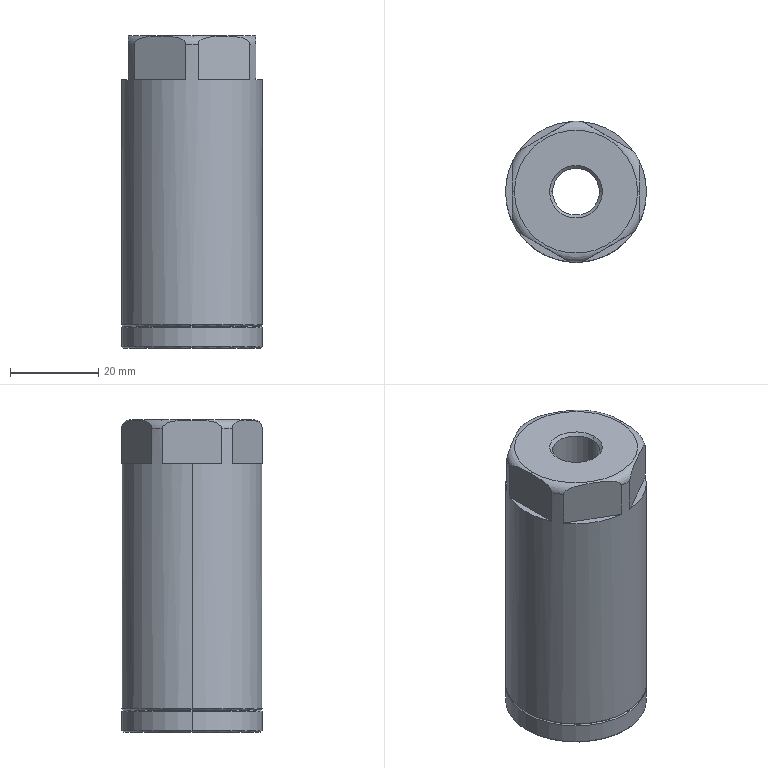Part | SolidWorks | features BaseBody 1 | 1 solid | 35 faces | box 32 x 32 x 71 mm | volume 42303 mm3 | plane 15 | cone 10 | cylinder 8 | torus 2 | commonest cylinder face diameters 10.647 x2 16.5 x2 31.9 x2 32 x2
STEP:
#1=CARTESIAN_POINT('',(-749.081,681.211,947.532));
#2=VERTEX_POINT('',#1);
#3=CARTESIAN_POINT('',(-717.181,681.211,947.532));
#4=VERTEX_POINT('',#3);
#5=CARTESIAN_POINT('',(-733.131,681.211,947.532));
#6=DIRECTION('',(0.,0.,1.));
#7=DIRECTION('',(-1.,0.,0.));
#8=AXIS2_PLACEMENT_3D('',#5,#6,#7);
#9=CIRCLE('',#8,15.95);
#10=EDGE_CURVE('',#2,#4,#9,.T.);
#11=ORIENTED_EDGE('',*,*,#10,.F.);
#12=CARTESIAN_POINT('',(-748.781,681.211,947.232));
#13=VERTEX_POINT('',#12);
#14=CARTESIAN_POINT('',(-748.781,681.211,947.232));
#15=DIRECTION('',(-0.7071,0.,0.7071));
#16=VECTOR('',#15,1000.);
#17=LINE('',#14,#16);
#18=EDGE_CURVE('',#13,#2,#17,.T.);
#19=ORIENTED_EDGE('',*,*,#18,.F.);
#20=CARTESIAN_POINT('',(-717.481,681.211,947.232));
#21=VERTEX_POINT('',#20);
#22=CARTESIAN_POINT('',(-733.131,681.211,947.232));
#23=DIRECTION('',(0.,0.,1.));
#24=DIRECTION('',(-1.,0.,0.));
#25=AXIS2_PLACEMENT_3D('',#22,#23,#24);
#26=CIRCLE('',#25,15.65);
#27=EDGE_CURVE('',#13,#21,#26,.T.);
#28=ORIENTED_EDGE('',*,*,#27,.T.);
#29=CARTESIAN_POINT('',(-717.181,681.211,947.532));
#30=DIRECTION('',(-0.7071,0.,-0.7071));
#31=VECTOR('',#30,1000.);
#32=LINE('',#29,#31);
#33=EDGE_CURVE('',#4,#21,#32,.T.);
#34=ORIENTED_EDGE('',*,*,#33,.F.);
#35=EDGE_LOOP('',(#11,#19,#28,#34));
#36=FACE_OUTER_BOUND('',#35,.T.);
#37=CARTESIAN_POINT('',(-733.131,681.211,947.382));
#38=DIRECTION('',(0.,0.,1.));
#39=DIRECTION('',(1.,0.,0.));
#40=AXIS2_PLACEMENT_3D('',#37,#38,#39);
#41=CONICAL_SURFACE('',#40,15.8,0.7854);
#42=ADVANCED_FACE('',(#36),#41,.T.);
#43=ORIENTED_EDGE('',*,*,#18,.T.);
#44=CARTESIAN_POINT('',(-733.131,681.211,947.532));
#45=DIRECTION('',(0.,0.,1.));
#46=DIRECTION('',(1.,0.,0.));
#47=AXIS2_PLACEMENT_3D('',#44,#45,#46);
#48=CIRCLE('',#47,15.95);
#49=EDGE_CURVE('',#4,#2,#48,.T.);
#50=ORIENTED_EDGE('',*,*,#49,.F.);
#51=ORIENTED_EDGE('',*,*,#33,.T.);
#52=CARTESIAN_POINT('',(-733.131,681.211,947.232));
#53=DIRECTION('',(0.,0.,1.));
#54=DIRECTION('',(1.,0.,0.));
#55=AXIS2_PLACEMENT_3D('',#52,#53,#54);
#56=CIRCLE('',#55,15.65);
#57=EDGE_CURVE('',#21,#13,#56,.T.);
#58=ORIENTED_EDGE('',*,*,#57,.T.);
#59=EDGE_LOOP('',(#43,#50,#51,#58));
#60=FACE_OUTER_BOUND('',#59,.T.);
#61=CARTESIAN_POINT('',(-733.131,681.211,947.382));
#62=DIRECTION('',(0.,0.,1.));
#63=DIRECTION('',(-1.,0.,0.));
#64=AXIS2_PLACEMENT_3D('',#61,#62,#63);
#65=CONICAL_SURFACE('',#64,15.8,0.7854);
#66=ADVANCED_FACE('',(#60),#65,.T.);
#67=ORIENTED_EDGE('',*,*,#27,.F.);
#68=ORIENTED_EDGE('',*,*,#57,.F.);
#69=EDGE_LOOP('',(#67,#68));
#70=FACE_OUTER_BOUND('',#69,.T.);
#71=CARTESIAN_POINT('',(-724.881,681.211,947.232));
#72=VERTEX_POINT('',#71);
#73=CARTESIAN_POINT('',(-741.381,681.211,947.232));
#74=VERTEX_POINT('',#73);
#75=CARTESIAN_POINT('',(-733.131,681.211,947.232));
#76=DIRECTION('',(0.,0.,-1.));
#77=DIRECTION('',(1.,0.,0.));
#78=AXIS2_PLACEMENT_3D('',#75,#76,#77);
#79=CIRCLE('',#78,8.25);
#80=EDGE_CURVE('',#72,#74,#79,.T.);
#81=ORIENTED_EDGE('',*,*,#80,.F.);
#82=CARTESIAN_POINT('',(-733.131,681.211,947.232));
#83=DIRECTION('',(0.,0.,-1.));
#84=DIRECTION('',(-1.,0.,0.));
#85=AXIS2_PLACEMENT_3D('',#82,#83,#84);
#86=CIRCLE('',#85,8.25);
#87=EDGE_CURVE('',#74,#72,#86,.T.);
#88=ORIENTED_EDGE('',*,*,#87,.F.);
#89=EDGE_LOOP('',(#81,#88));
#90=FACE_BOUND('',#89,.T.);
#91=CARTESIAN_POINT('',(-733.131,665.561,947.232));
#92=DIRECTION('',(0.,0.,1.));
#93=DIRECTION('',(1.,0.,0.));
#94=AXIS2_PLACEMENT_3D('',#91,#92,#93);
#95=PLANE('',#94);
#96=ADVANCED_FACE('',(#70,#90),#95,.F.);
#97=CARTESIAN_POINT('',(-724.881,681.211,1007.232));
#98=VERTEX_POINT('',#97);
#99=CARTESIAN_POINT('',(-741.381,681.211,1007.232));
#100=VERTEX_POINT('',#99);
#101=CARTESIAN_POINT('',(-733.131,681.211,1007.232));
#102=DIRECTION('',(0.,0.,1.));
#103=DIRECTION('',(1.,0.,0.));
#104=AXIS2_PLACEMENT_3D('',#101,#102,#103);
#105=CIRCLE('',#104,8.25);
#106=EDGE_CURVE('',#98,#100,#105,.T.);
#107=ORIENTED_EDGE('',*,*,#106,.T.);
#108=CARTESIAN_POINT('',(-741.381,681.211,1007.232));
#109=DIRECTION('',(0.,0.,-1.));
#110=VECTOR('',#109,1000.);
#111=LINE('',#108,#110);
#112=EDGE_CURVE('',#100,#74,#111,.T.);
#113=ORIENTED_EDGE('',*,*,#112,.T.);
#114=ORIENTED_EDGE('',*,*,#87,.T.);
#115=CARTESIAN_POINT('',(-724.881,681.211,947.232));
#116=DIRECTION('',(0.,0.,1.));
#117=VECTOR('',#116,1000.);
#118=LINE('',#115,#117);
#119=EDGE_CURVE('',#72,#98,#118,.T.);
#120=ORIENTED_EDGE('',*,*,#119,.T.);
#121=EDGE_LOOP('',(#107,#113,#114,#120));
#122=FACE_OUTER_BOUND('',#121,.T.);
#123=CARTESIAN_POINT('',(-733.131,681.211,947.232));
#124=DIRECTION('',(0.,0.,1.));
#125=DIRECTION('',(1.,0.,0.));
#126=AXIS2_PLACEMENT_3D('',#123,#124,#125);
#127=CYLINDRICAL_SURFACE('',#126,8.25);
#128=ADVANCED_FACE('',(#122),#127,.F.);
#129=ORIENTED_EDGE('',*,*,#112,.F.);
#130=CARTESIAN_POINT('',(-733.131,681.211,1007.232));
#131=DIRECTION('',(0.,0.,1.));
#132=DIRECTION('',(-1.,0.,0.));
#133=AXIS2_PLACEMENT_3D('',#130,#131,#132);
#134=CIRCLE('',#133,8.25);
#135=EDGE_CURVE('',#100,#98,#134,.T.);
#136=ORIENTED_EDGE('',*,*,#135,.T.);
#137=ORIENTED_EDGE('',*,*,#119,.F.);
#138=ORIENTED_EDGE('',*,*,#80,.T.);
#139=EDGE_LOOP('',(#129,#136,#137,#138));
#140=FACE_OUTER_BOUND('',#139,.T.);
#141=CARTESIAN_POINT('',(-733.131,681.211,947.232));
#142=DIRECTION('',(0.,0.,1.));
#143=DIRECTION('',(1.,0.,0.));
#144=AXIS2_PLACEMENT_3D('',#141,#142,#143);
#145=CYLINDRICAL_SURFACE('',#144,8.25);
#146=ADVANCED_FACE('',(#140),#145,.F.);
#147=CARTESIAN_POINT('',(-727.807,681.211,1008.921));
#148=VERTEX_POINT('',#147);
#149=CARTESIAN_POINT('',(-727.807,681.211,1008.921));
#150=DIRECTION('',(0.866,0.,-0.5));
#151=VECTOR('',#150,1000.);
#152=LINE('',#149,#151);
#153=EDGE_CURVE('',#148,#98,#152,.T.);
#154=ORIENTED_EDGE('',*,*,#153,.T.);
#155=ORIENTED_EDGE('',*,*,#135,.F.);
#156=CARTESIAN_POINT('',(-738.454,681.211,1008.921));
#157=VERTEX_POINT('',#156);
#158=CARTESIAN_POINT('',(-741.381,681.211,1007.232));
#159=DIRECTION('',(0.866,0.,0.5));
#160=VECTOR('',#159,1000.);
#161=LINE('',#158,#160);
#162=EDGE_CURVE('',#100,#157,#161,.T.);
#163=ORIENTED_EDGE('',*,*,#162,.T.);
#164=CARTESIAN_POINT('',(-733.131,681.211,1008.921));
#165=DIRECTION('',(0.,0.,-1.));
#166=DIRECTION('',(1.,0.,0.));
#167=AXIS2_PLACEMENT_3D('',#164,#165,#166);
#168=CIRCLE('',#167,5.323);
#169=EDGE_CURVE('',#148,#157,#168,.T.);
#170=ORIENTED_EDGE('',*,*,#169,.F.);
#171=EDGE_LOOP('',(#154,#155,#163,#170));
#172=FACE_OUTER_BOUND('',#171,.T.);
#173=CARTESIAN_POINT('',(-733.131,681.211,1008.077));
#174=DIRECTION('',(0.,0.,-1.));
#175=DIRECTION('',(1.,0.,0.));
#176=AXIS2_PLACEMENT_3D('',#173,#174,#175);
#177=CONICAL_SURFACE('',#176,6.787,1.047);
#178=ADVANCED_FACE('',(#172),#177,.F.);
#179=CARTESIAN_POINT('',(-738.454,681.211,1017.555));
#180=VERTEX_POINT('',#179);
#181=CARTESIAN_POINT('',(-738.454,681.211,1008.921));
#182=DIRECTION('',(0.,0.,1.));
#183=VECTOR('',#182,1000.);
#184=LINE('',#181,#183);
#185=EDGE_CURVE('',#157,#180,#184,.T.);
#186=ORIENTED_EDGE('',*,*,#185,.T.);
#187=CARTESIAN_POINT('',(-727.807,681.211,1017.555));
#188=VERTEX_POINT('',#187);
#189=CARTESIAN_POINT('',(-733.131,681.211,1017.555));
#190=DIRECTION('',(0.,0.,1.));
#191=DIRECTION('',(-1.,0.,0.));
#192=AXIS2_PLACEMENT_3D('',#189,#190,#191);
#193=CIRCLE('',#192,5.324);
#194=EDGE_CURVE('',#180,#188,#193,.T.);
#195=ORIENTED_EDGE('',*,*,#194,.T.);
#196=CARTESIAN_POINT('',(-727.807,681.211,1017.555));
#197=DIRECTION('',(0.,0.,-1.));
#198=VECTOR('',#197,1000.);
#199=LINE('',#196,#198);
#200=EDGE_CURVE('',#188,#148,#199,.T.);
#201=ORIENTED_EDGE('',*,*,#200,.T.);
#202=ORIENTED_EDGE('',*,*,#169,.T.);
#203=EDGE_LOOP('',(#186,#195,#201,#202));
#204=FACE_OUTER_BOUND('',#203,.T.);
#205=CARTESIAN_POINT('',(-733.131,681.211,947.232));
#206=DIRECTION('',(0.,0.,1.));
#207=DIRECTION('',(1.,0.,0.));
#208=AXIS2_PLACEMENT_3D('',#205,#206,#207);
#209=CYLINDRICAL_SURFACE('',#208,5.324);
#210=ADVANCED_FACE('',(#204),#209,.F.);
#211=CARTESIAN_POINT('',(-733.131,681.211,1017.555));
#212=DIRECTION('',(0.,0.,1.));
#213=DIRECTION('',(1.,0.,0.));
#214=AXIS2_PLACEMENT_3D('',#211,#212,#213);
#215=CIRCLE('',#214,5.324);
#216=EDGE_CURVE('',#188,#180,#215,.T.);
#217=ORIENTED_EDGE('',*,*,#216,.T.);
#218=ORIENTED_EDGE('',*,*,#185,.F.);
#219=CARTESIAN_POINT('',(-733.131,681.211,1008.921));
#220=DIRECTION('',(0.,0.,-1.));
#221=DIRECTION('',(-1.,0.,0.));
#222=AXIS2_PLACEMENT_3D('',#219,#220,#221);
#223=CIRCLE('',#222,5.323);
#224=EDGE_CURVE('',#157,#148,#223,.T.);
#225=ORIENTED_EDGE('',*,*,#224,.T.);
#226=ORIENTED_EDGE('',*,*,#200,.F.);
#227=EDGE_LOOP('',(#217,#218,#225,#226));
#228=FACE_OUTER_BOUND('',#227,.T.);
#229=CARTESIAN_POINT('',(-733.131,681.211,947.232));
#230=DIRECTION('',(0.,0.,1.));
#231=DIRECTION('',(1.,0.,0.));
#232=AXIS2_PLACEMENT_3D('',#229,#230,#231);
#233=CYLINDRICAL_SURFACE('',#232,5.324);
#234=ADVANCED_FACE('',(#228),#233,.F.);
#235=ORIENTED_EDGE('',*,*,#106,.F.);
#236=ORIENTED_EDGE('',*,*,#153,.F.);
#237=ORIENTED_EDGE('',*,*,#224,.F.);
#238=ORIENTED_EDGE('',*,*,#162,.F.);
#239=EDGE_LOOP('',(#235,#236,#237,#238));
#240=FACE_OUTER_BOUND('',#239,.T.);
#241=CARTESIAN_POINT('',(-733.131,681.211,1008.077));
#242=DIRECTION('',(0.,0.,-1.));
#243=DIRECTION('',(1.,0.,0.));
#244=AXIS2_PLACEMENT_3D('',#241,#242,#243);
#245=CONICAL_SURFACE('',#244,6.787,1.047);
#246=ADVANCED_FACE('',(#240),#245,.F.);
#247=CARTESIAN_POINT('',(-727.131,681.211,1018.232));
#248=VERTEX_POINT('',#247);
#249=CARTESIAN_POINT('',(-739.131,681.211,1018.232));
#250=VERTEX_POINT('',#249);
#251=CARTESIAN_POINT('',(-733.131,681.211,1018.232));
#252=DIRECTION('',(0.,0.,1.));
#253=DIRECTION('',(1.,0.,0.));
#254=AXIS2_PLACEMENT_3D('',#251,#252,#253);
#255=CIRCLE('',#254,6.);
#256=EDGE_CURVE('',#248,#250,#255,.T.);
#257=ORIENTED_EDGE('',*,*,#256,.T.);
#258=CARTESIAN_POINT('',(-739.131,681.211,1018.232));
#259=DIRECTION('',(0.7071,0.,-0.7071));
#260=VECTOR('',#259,1000.);
#261=LINE('',#258,#260);
#262=EDGE_CURVE('',#250,#180,#261,.T.);
#263=ORIENTED_EDGE('',*,*,#262,.T.);
#264=ORIENTED_EDGE('',*,*,#216,.F.);
#265=CARTESIAN_POINT('',(-727.807,681.211,1017.555));
#266=DIRECTION('',(0.7071,0.,0.7071));
#267=VECTOR('',#266,1000.);
#268=LINE('',#265,#267);
#269=EDGE_CURVE('',#188,#248,#268,.T.);
#270=ORIENTED_EDGE('',*,*,#269,.T.);
#271=EDGE_LOOP('',(#257,#263,#264,#270));
#272=FACE_OUTER_BOUND('',#271,.T.);
#273=CARTESIAN_POINT('',(-733.131,681.211,1017.893));
#274=DIRECTION('',(0.,0.,1.));
#275=DIRECTION('',(-1.,0.,0.));
#276=AXIS2_PLACEMENT_3D('',#273,#274,#275);
#277=CONICAL_SURFACE('',#276,5.662,0.7854);
#278=ADVANCED_FACE('',(#272),#277,.F.);
#279=ORIENTED_EDGE('',*,*,#262,.F.);
#280=CARTESIAN_POINT('',(-733.131,681.211,1018.232));
#281=DIRECTION('',(0.,0.,1.));
#282=DIRECTION('',(-1.,0.,0.));
#283=AXIS2_PLACEMENT_3D('',#280,#281,#282);
#284=CIRCLE('',#283,6.);
#285=EDGE_CURVE('',#250,#248,#284,.T.);
#286=ORIENTED_EDGE('',*,*,#285,.T.);
#287=ORIENTED_EDGE('',*,*,#269,.F.);
#288=ORIENTED_EDGE('',*,*,#194,.F.);
#289=EDGE_LOOP('',(#279,#286,#287,#288));
#290=FACE_OUTER_BOUND('',#289,.T.);
#291=CARTESIAN_POINT('',(-733.131,681.211,1017.893));
#292=DIRECTION('',(0.,0.,1.));
#293=DIRECTION('',(-1.,0.,0.));
#294=AXIS2_PLACEMENT_3D('',#291,#292,#293);
#295=CONICAL_SURFACE('',#294,5.662,0.7854);
#296=ADVANCED_FACE('',(#290),#295,.F.);
#297=CARTESIAN_POINT('',(-719.131,681.211,1018.232));
#298=VERTEX_POINT('',#297);
#299=CARTESIAN_POINT('',(-747.131,681.211,1018.232));
#300=VERTEX_POINT('',#299);
#301=CARTESIAN_POINT('',(-733.131,681.211,1018.232));
#302=DIRECTION('',(0.,0.,-1.));
#303=DIRECTION('',(1.,0.,0.));
#304=AXIS2_PLACEMENT_3D('',#301,#302,#303);
#305=CIRCLE('',#304,14.);
#306=EDGE_CURVE('',#298,#300,#305,.T.);
#307=ORIENTED_EDGE('',*,*,#306,.F.);
#308=CARTESIAN_POINT('',(-733.131,681.211,1018.232));
#309=DIRECTION('',(0.,0.,-1.));
#310=DIRECTION('',(-1.,0.,0.));
#311=AXIS2_PLACEMENT_3D('',#308,#309,#310);
#312=CIRCLE('',#311,14.);
#313=EDGE_CURVE('',#300,#298,#312,.T.);
#314=ORIENTED_EDGE('',*,*,#313,.F.);
#315=EDGE_LOOP('',(#307,#314));
#316=FACE_OUTER_BOUND('',#315,.T.);
#317=ORIENTED_EDGE('',*,*,#285,.F.);
#318=ORIENTED_EDGE('',*,*,#256,.F.);
#319=EDGE_LOOP('',(#317,#318));
#320=FACE_BOUND('',#319,.T.);
#321=CARTESIAN_POINT('',(-733.131,681.211,1018.232));
#322=DIRECTION('',(0.,0.,-1.));
#323=DIRECTION('',(-1.,0.,0.));
#324=AXIS2_PLACEMENT_3D('',#321,#322,#323);
#325=PLANE('',#324);
#326=ADVANCED_FACE('',(#316,#320),#325,.F.);
#327=CARTESIAN_POINT('',(-720.023,690.386,1016.232));
#328=VERTEX_POINT('',#327);
#329=CARTESIAN_POINT('',(-718.631,687.974,1016.232));
#330=VERTEX_POINT('',#329);
#331=CARTESIAN_POINT('',(-733.131,681.211,1016.232));
#332=DIRECTION('',(0.,0.,-1.));
#333=DIRECTION('',(0.8192,0.5735,0.));
#334=AXIS2_PLACEMENT_3D('',#331,#332,#333);
#335=CIRCLE('',#334,16.);
#336=EDGE_CURVE('',#328,#330,#335,.T.);
#337=ORIENTED_EDGE('',*,*,#336,.F.);
#338=CARTESIAN_POINT('',(-731.738,697.15,1016.232));
#339=VERTEX_POINT('',#338);
#340=CARTESIAN_POINT('',(-731.738,697.15,1016.232));
#341=CARTESIAN_POINT('',(-731.738,697.15,1016.391));
#342=CARTESIAN_POINT('',(-731.698,697.127,1016.546));
#343=CARTESIAN_POINT('',(-731.565,697.05,1016.822));
#344=CARTESIAN_POINT('',(-731.474,696.997,1016.943));
#345=CARTESIAN_POINT('',(-731.271,696.88,1017.152));
#346=CARTESIAN_POINT('',(-731.158,696.815,1017.243));
#347=CARTESIAN_POINT('',(-730.924,696.68,1017.401));
#348=CARTESIAN_POINT('',(-730.802,696.609,1017.469));
#349=CARTESIAN_POINT('',(-730.426,696.392,1017.651));
#350=CARTESIAN_POINT('',(-730.165,696.241,1017.741));
#351=CARTESIAN_POINT('',(-729.641,695.939,1017.884));
#352=CARTESIAN_POINT('',(-729.377,695.787,1017.937));
#353=CARTESIAN_POINT('',(-728.579,695.326,1018.065));
#354=CARTESIAN_POINT('',(-728.04,695.015,1018.107));
#355=CARTESIAN_POINT('',(-726.964,694.393,1018.159));
#356=CARTESIAN_POINT('',(-726.426,694.083,1018.168));
#357=CARTESIAN_POINT('',(-725.351,693.462,1018.168));
#358=CARTESIAN_POINT('',(-724.814,693.152,1018.159));
#359=CARTESIAN_POINT('',(-723.741,692.533,1018.108));
#360=CARTESIAN_POINT('',(-723.205,692.223,1018.067));
#361=CARTESIAN_POINT('',(-722.404,691.761,1017.941));
#362=CARTESIAN_POINT('',(-722.137,691.607,1017.888));
#363=CARTESIAN_POINT('',(-721.605,691.3,1017.744));
#364=CARTESIAN_POINT('',(-721.342,691.148,1017.654));
#365=CARTESIAN_POINT('',(-720.964,690.929,1017.472));
#366=CARTESIAN_POINT('',(-720.842,690.859,1017.404));
#367=CARTESIAN_POINT('',(-720.608,690.724,1017.247));
#368=CARTESIAN_POINT('',(-720.497,690.66,1017.159));
#369=CARTESIAN_POINT('',(-720.292,690.541,1016.948));
#370=CARTESIAN_POINT('',(-720.199,690.488,1016.826));
#371=CARTESIAN_POINT('',(-720.098,690.429,1016.617));
#372=CARTESIAN_POINT('',(-720.071,690.413,1016.545));
#373=CARTESIAN_POINT('',(-720.033,690.392,1016.393));
#374=CARTESIAN_POINT('',(-720.023,690.386,1016.312));
#375=CARTESIAN_POINT('',(-720.023,690.386,1016.232));
#376=B_SPLINE_CURVE_WITH_KNOTS('',3,(#340,#341,#342,#343,#344,#345,#346,#347,#348,#349,#350,#351,#352,#353,#354,#355,#356,#357,#358,#359,#360,#361,#362,#363,#364,#365,#366,#367,#368,#369,#370,#371,#372,#373,#374,#375),.UNSPECIFIED.,.F.,.F.,(4,2,2,2,2,2,2,2,2,2,2,2,2,2,2,2,2,4),(0.,0.0004713,0.0009425,0.001414,0.001885,0.002828,0.00377,0.005655,0.00754,0.009425,0.01131,0.01225,0.0132,0.01367,0.01414,0.01461,0.01484,0.01508),.UNSPECIFIED.);
#377=EDGE_CURVE('',#339,#328,#376,.T.);
#378=ORIENTED_EDGE('',*,*,#377,.F.);
#379=CARTESIAN_POINT('',(-734.523,697.15,1016.232));
#380=VERTEX_POINT('',#379);
#381=CARTESIAN_POINT('',(-733.131,681.211,1016.232));
#382=DIRECTION('',(0.,0.,-1.));
#383=DIRECTION('',(-0.08702,0.9962,0.));
#384=AXIS2_PLACEMENT_3D('',#381,#382,#383);
#385=CIRCLE('',#384,16.);
#386=EDGE_CURVE('',#380,#339,#385,.T.);
#387=ORIENTED_EDGE('',*,*,#386,.F.);
#388=CARTESIAN_POINT('',(-746.238,690.386,1016.232));
#389=VERTEX_POINT('',#388);
#390=CARTESIAN_POINT('',(-746.238,690.386,1016.232));
#391=CARTESIAN_POINT('',(-746.238,690.386,1016.391));
#392=CARTESIAN_POINT('',(-746.198,690.409,1016.546));
#393=CARTESIAN_POINT('',(-746.065,690.486,1016.822));
#394=CARTESIAN_POINT('',(-745.974,690.539,1016.943));
#395=CARTESIAN_POINT('',(-745.771,690.656,1017.152));
#396=CARTESIAN_POINT('',(-745.658,690.721,1017.243));
#397=CARTESIAN_POINT('',(-745.424,690.856,1017.401));
#398=CARTESIAN_POINT('',(-745.302,690.927,1017.469));
#399=CARTESIAN_POINT('',(-744.926,691.143,1017.651));
#400=CARTESIAN_POINT('',(-744.665,691.295,1017.741));
#401=CARTESIAN_POINT('',(-744.141,691.597,1017.884));
#402=CARTESIAN_POINT('',(-743.877,691.749,1017.937));
#403=CARTESIAN_POINT('',(-743.079,692.21,1018.065));
#404=CARTESIAN_POINT('',(-742.54,692.521,1018.107));
#405=CARTESIAN_POINT('',(-741.464,693.143,1018.159));
#406=CARTESIAN_POINT('',(-740.926,693.453,1018.168));
#407=CARTESIAN_POINT('',(-739.851,694.074,1018.168));
#408=CARTESIAN_POINT('',(-739.314,694.384,1018.159));
#409=CARTESIAN_POINT('',(-738.241,695.003,1018.108));
#410=CARTESIAN_POINT('',(-737.705,695.313,1018.067));
#411=CARTESIAN_POINT('',(-736.904,695.775,1017.941));
#412=CARTESIAN_POINT('',(-736.637,695.929,1017.888));
#413=CARTESIAN_POINT('',(-736.105,696.236,1017.744));
#414=CARTESIAN_POINT('',(-735.842,696.388,1017.654));
#415=CARTESIAN_POINT('',(-735.464,696.606,1017.472));
#416=CARTESIAN_POINT('',(-735.342,696.677,1017.404));
#417=CARTESIAN_POINT('',(-735.108,696.812,1017.247));
#418=CARTESIAN_POINT('',(-734.997,696.876,1017.159));
#419=CARTESIAN_POINT('',(-734.792,696.995,1016.948));
#420=CARTESIAN_POINT('',(-734.699,697.048,1016.826));
#421=CARTESIAN_POINT('',(-734.598,697.107,1016.617));
#422=CARTESIAN_POINT('',(-734.571,697.122,1016.545));
#423=CARTESIAN_POINT('',(-734.533,697.144,1016.393));
#424=CARTESIAN_POINT('',(-734.523,697.15,1016.312));
#425=CARTESIAN_POINT('',(-734.523,697.15,1016.232));
#426=B_SPLINE_CURVE_WITH_KNOTS('',3,(#390,#391,#392,#393,#394,#395,#396,#397,#398,#399,#400,#401,#402,#403,#404,#405,#406,#407,#408,#409,#410,#411,#412,#413,#414,#415,#416,#417,#418,#419,#420,#421,#422,#423,#424,#425),.UNSPECIFIED.,.F.,.F.,(4,2,2,2,2,2,2,2,2,2,2,2,2,2,2,2,2,4),(0.,0.0004713,0.0009425,0.001414,0.001885,0.002828,0.00377,0.005655,0.00754,0.009425,0.01131,0.01225,0.0132,0.01367,0.01414,0.01461,0.01484,0.01508),.UNSPECIFIED.);
#427=EDGE_CURVE('',#389,#380,#426,.T.);
#428=ORIENTED_EDGE('',*,*,#427,.F.);
#429=CARTESIAN_POINT('',(-747.631,687.974,1016.232));
#430=VERTEX_POINT('',#429);
#431=CARTESIAN_POINT('',(-733.131,681.211,1016.232));
#432=DIRECTION('',(0.,0.,-1.));
#433=DIRECTION('',(-0.9063,0.4227,0.));
#434=AXIS2_PLACEMENT_3D('',#431,#432,#433);
#435=CIRCLE('',#434,16.);
#436=EDGE_CURVE('',#430,#389,#435,.T.);
#437=ORIENTED_EDGE('',*,*,#436,.F.);
#438=CARTESIAN_POINT('',(-747.631,681.211,1018.168));
#439=VERTEX_POINT('',#438);
#440=CARTESIAN_POINT('',(-747.631,687.974,1016.232));
#441=CARTESIAN_POINT('',(-747.631,687.974,1016.278));
#442=CARTESIAN_POINT('',(-747.631,687.967,1016.372));
#443=CARTESIAN_POINT('',(-747.631,687.931,1016.515));
#444=CARTESIAN_POINT('',(-747.631,687.868,1016.662));
#445=CARTESIAN_POINT('',(-747.631,687.773,1016.813));
#446=CARTESIAN_POINT('',(-747.631,687.642,1016.967));
#447=CARTESIAN_POINT('',(-747.631,687.471,1017.122));
#448=CARTESIAN_POINT('',(-747.631,687.259,1017.273));
#449=CARTESIAN_POINT('',(-747.631,687.001,1017.419));
#450=CARTESIAN_POINT('',(-747.631,686.697,1017.556));
#451=CARTESIAN_POINT('',(-747.631,686.345,1017.682));
#452=CARTESIAN_POINT('',(-747.631,685.942,1017.795));
#453=CARTESIAN_POINT('',(-747.631,685.486,1017.895));
#454=CARTESIAN_POINT('',(-747.631,684.969,1017.98));
#455=CARTESIAN_POINT('',(-747.631,684.388,1018.049));
#456=CARTESIAN_POINT('',(-747.631,683.735,1018.102));
#457=CARTESIAN_POINT('',(-747.631,682.999,1018.14));
#458=CARTESIAN_POINT('',(-747.631,682.171,1018.162));
#459=CARTESIAN_POINT('',(-747.631,681.543,1018.168));
#460=CARTESIAN_POINT('',(-747.631,681.211,1018.168));
#461=B_SPLINE_CURVE_WITH_KNOTS('',3,(#440,#441,#442,#443,#444,#445,#446,#447,#448,#449,#450,#451,#452,#453,#454,#455,#456,#457,#458,#459,#460),.UNSPECIFIED.,.F.,.F.,(4,1,1,1,1,1,1,1,1,1,1,1,1,1,1,1,1,1,4),(0.,0.05556,0.1111,0.1667,0.2222,0.2778,0.3333,0.3889,0.4444,0.5,0.5556,0.6111,0.6667,0.7222,0.7778,0.8333,0.8889,0.9444,1.),.UNSPECIFIED.);
#462=EDGE_CURVE('',#430,#439,#461,.T.);
#463=ORIENTED_EDGE('',*,*,#462,.T.);
#464=CARTESIAN_POINT('',(-747.131,681.211,1016.232));
#465=DIRECTION('',(0.,-1.,0.));
#466=DIRECTION('',(0.,0.,1.));
#467=AXIS2_PLACEMENT_3D('',#464,#465,#466);
#468=CIRCLE('',#467,2.);
#469=EDGE_CURVE('',#300,#439,#468,.T.);
#470=ORIENTED_EDGE('',*,*,#469,.F.);
#471=ORIENTED_EDGE('',*,*,#313,.T.);
#472=CARTESIAN_POINT('',(-718.631,681.211,1018.168));
#473=VERTEX_POINT('',#472);
#474=CARTESIAN_POINT('',(-719.131,681.211,1016.232));
#475=DIRECTION('',(0.,-1.,0.));
#476=DIRECTION('',(0.25,0.,0.9682));
#477=AXIS2_PLACEMENT_3D('',#474,#475,#476);
#478=CIRCLE('',#477,2.);
#479=EDGE_CURVE('',#473,#298,#478,.T.);
#480=ORIENTED_EDGE('',*,*,#479,.F.);
#481=CARTESIAN_POINT('',(-718.631,687.974,1016.232));
#482=CARTESIAN_POINT('',(-718.631,687.974,1016.278));
#483=CARTESIAN_POINT('',(-718.631,687.967,1016.372));
#484=CARTESIAN_POINT('',(-718.631,687.931,1016.515));
#485=CARTESIAN_POINT('',(-718.631,687.868,1016.662));
#486=CARTESIAN_POINT('',(-718.631,687.773,1016.813));
#487=CARTESIAN_POINT('',(-718.631,687.643,1016.967));
#488=CARTESIAN_POINT('',(-718.631,687.471,1017.122));
#489=CARTESIAN_POINT('',(-718.631,687.259,1017.273));
#490=CARTESIAN_POINT('',(-718.631,687.001,1017.419));
#491=CARTESIAN_POINT('',(-718.631,686.697,1017.556));
#492=CARTESIAN_POINT('',(-718.631,686.345,1017.682));
#493=CARTESIAN_POINT('',(-718.631,685.942,1017.795));
#494=CARTESIAN_POINT('',(-718.631,685.486,1017.895));
#495=CARTESIAN_POINT('',(-718.631,684.969,1017.98));
#496=CARTESIAN_POINT('',(-718.631,684.388,1018.049));
#497=CARTESIAN_POINT('',(-718.631,683.735,1018.102));
#498=CARTESIAN_POINT('',(-718.631,682.999,1018.14));
#499=CARTESIAN_POINT('',(-718.631,682.171,1018.162));
#500=CARTESIAN_POINT('',(-718.631,681.543,1018.168));
#501=CARTESIAN_POINT('',(-718.631,681.211,1018.168));
#502=B_SPLINE_CURVE_WITH_KNOTS('',3,(#481,#482,#483,#484,#485,#486,#487,#488,#489,#490,#491,#492,#493,#494,#495,#496,#497,#498,#499,#500,#501),.UNSPECIFIED.,.F.,.F.,(4,1,1,1,1,1,1,1,1,1,1,1,1,1,1,1,1,1,4),(0.,0.05556,0.1111,0.1667,0.2222,0.2778,0.3333,0.3889,0.4444,0.5,0.5556,0.6111,0.6667,0.7222,0.7778,0.8333,0.8889,0.9444,1.),.UNSPECIFIED.);
#503=EDGE_CURVE('',#330,#473,#502,.T.);
#504=ORIENTED_EDGE('',*,*,#503,.F.);
#505=EDGE_LOOP('',(#337,#378,#387,#428,#437,#463,#470,#471,#480,#504));
#506=FACE_OUTER_BOUND('',#505,.T.);
#507=CARTESIAN_POINT('',(-733.131,681.211,1016.232));
#508=DIRECTION('',(0.,0.,1.));
#509=DIRECTION('',(1.,0.,0.));
#510=AXIS2_PLACEMENT_3D('',#507,#508,#509);
#511=TOROIDAL_SURFACE('',#510,14.,2.);
#512=ADVANCED_FACE('',(#506),#511,.T.);
#513=ORIENTED_EDGE('',*,*,#503,.T.);
#514=CARTESIAN_POINT('',(-718.631,674.447,1016.232));
#515=VERTEX_POINT('',#514);
#516=CARTESIAN_POINT('',(-718.631,674.447,1016.232));
#517=CARTESIAN_POINT('',(-718.631,674.447,1016.278));
#518=CARTESIAN_POINT('',(-718.631,674.454,1016.372));
#519=CARTESIAN_POINT('',(-718.631,674.49,1016.515));
#520=CARTESIAN_POINT('',(-718.631,674.553,1016.662));
#521=CARTESIAN_POINT('',(-718.631,674.648,1016.813));
#522=CARTESIAN_POINT('',(-718.631,674.779,1016.967));
#523=CARTESIAN_POINT('',(-718.631,674.95,1017.122));
#524=CARTESIAN_POINT('',(-718.631,675.162,1017.273));
#525=CARTESIAN_POINT('',(-718.631,675.42,1017.419));
#526=CARTESIAN_POINT('',(-718.631,675.724,1017.556));
#527=CARTESIAN_POINT('',(-718.631,676.076,1017.682));
#528=CARTESIAN_POINT('',(-718.631,676.479,1017.795));
#529=CARTESIAN_POINT('',(-718.631,676.935,1017.895));
#530=CARTESIAN_POINT('',(-718.631,677.452,1017.98));
#531=CARTESIAN_POINT('',(-718.631,678.033,1018.049));
#532=CARTESIAN_POINT('',(-718.631,678.686,1018.102));
#533=CARTESIAN_POINT('',(-718.631,679.422,1018.14));
#534=CARTESIAN_POINT('',(-718.631,680.25,1018.162));
#535=CARTESIAN_POINT('',(-718.631,680.878,1018.168));
#536=CARTESIAN_POINT('',(-718.631,681.211,1018.168));
#537=B_SPLINE_CURVE_WITH_KNOTS('',3,(#516,#517,#518,#519,#520,#521,#522,#523,#524,#525,#526,#527,#528,#529,#530,#531,#532,#533,#534,#535,#536),.UNSPECIFIED.,.F.,.F.,(4,1,1,1,1,1,1,1,1,1,1,1,1,1,1,1,1,1,4),(0.,0.05556,0.1111,0.1667,0.2222,0.2778,0.3333,0.3889,0.4444,0.5,0.5556,0.6111,0.6667,0.7222,0.7778,0.8333,0.8889,0.9444,1.),.UNSPECIFIED.);
#538=EDGE_CURVE('',#515,#473,#537,.T.);
#539=ORIENTED_EDGE('',*,*,#538,.F.);
#540=CARTESIAN_POINT('',(-718.631,674.447,1008.232));
#541=VERTEX_POINT('',#540);
#542=CARTESIAN_POINT('',(-718.631,674.447,1016.232));
#543=DIRECTION('',(0.,0.,-1.));
#544=VECTOR('',#543,1000.);
#545=LINE('',#542,#544);
#546=EDGE_CURVE('',#515,#541,#545,.T.);
#547=ORIENTED_EDGE('',*,*,#546,.T.);
#548=CARTESIAN_POINT('',(-718.631,687.974,1008.232));
#549=VERTEX_POINT('',#548);
#550=CARTESIAN_POINT('',(-718.631,687.974,1008.232));
#551=DIRECTION('',(0.,-1.,0.));
#552=VECTOR('',#551,1000.);
#553=LINE('',#550,#552);
#554=EDGE_CURVE('',#549,#541,#553,.T.);
#555=ORIENTED_EDGE('',*,*,#554,.F.);
#556=CARTESIAN_POINT('',(-718.631,687.974,1008.232));
#557=DIRECTION('',(0.,0.,1.));
#558=VECTOR('',#557,1000.);
#559=LINE('',#556,#558);
#560=EDGE_CURVE('',#549,#330,#559,.T.);
#561=ORIENTED_EDGE('',*,*,#560,.T.);
#562=EDGE_LOOP('',(#513,#539,#547,#555,#561));
#563=FACE_OUTER_BOUND('',#562,.T.);
#564=CARTESIAN_POINT('',(-718.631,689.582,1008.232));
#565=DIRECTION('',(-1.,0.,0.));
#566=DIRECTION('',(0.,0.,1.));
#567=AXIS2_PLACEMENT_3D('',#564,#565,#566);
#568=PLANE('',#567);
#569=ADVANCED_FACE('',(#563),#568,.F.);
#570=CARTESIAN_POINT('',(-749.131,681.211,1008.232));
#571=VERTEX_POINT('',#570);
#572=CARTESIAN_POINT('',(-749.131,681.211,952.532));
#573=VERTEX_POINT('',#572);
#574=CARTESIAN_POINT('',(-749.131,681.211,1008.232));
#575=DIRECTION('',(0.,0.,-1.));
#576=VECTOR('',#575,1000.);
#577=LINE('',#574,#576);
#578=EDGE_CURVE('',#571,#573,#577,.T.);
#579=ORIENTED_EDGE('',*,*,#578,.F.);
#580=CARTESIAN_POINT('',(-747.631,687.974,1008.232));
#581=VERTEX_POINT('',#580);
#582=CARTESIAN_POINT('',(-733.131,681.211,1008.232));
#583=DIRECTION('',(0.,0.,-1.));
#584=DIRECTION('',(-1.,0.,0.));
#585=AXIS2_PLACEMENT_3D('',#582,#583,#584);
#586=CIRCLE('',#585,16.);
#587=EDGE_CURVE('',#571,#581,#586,.T.);
#588=ORIENTED_EDGE('',*,*,#587,.T.);
#589=CARTESIAN_POINT('',(-747.631,687.974,1016.232));
#590=DIRECTION('',(0.,0.,-1.));
#591=VECTOR('',#590,1000.);
#592=LINE('',#589,#591);
#593=EDGE_CURVE('',#430,#581,#592,.T.);
#594=ORIENTED_EDGE('',*,*,#593,.F.);
#595=ORIENTED_EDGE('',*,*,#436,.T.);
#596=CARTESIAN_POINT('',(-746.238,690.386,1008.232));
#597=VERTEX_POINT('',#596);
#598=CARTESIAN_POINT('',(-746.238,690.386,1008.232));
#599=DIRECTION('',(0.,0.,1.));
#600=VECTOR('',#599,1000.);
#601=LINE('',#598,#600);
#602=EDGE_CURVE('',#597,#389,#601,.T.);
#603=ORIENTED_EDGE('',*,*,#602,.F.);
#604=CARTESIAN_POINT('',(-734.523,697.15,1008.232));
#605=VERTEX_POINT('',#604);
#606=CARTESIAN_POINT('',(-733.131,681.211,1008.232));
#607=DIRECTION('',(0.,0.,-1.));
#608=DIRECTION('',(-0.8192,0.5735,0.));
#609=AXIS2_PLACEMENT_3D('',#606,#607,#608);
#610=CIRCLE('',#609,16.);
#611=EDGE_CURVE('',#597,#605,#610,.T.);
#612=ORIENTED_EDGE('',*,*,#611,.T.);
#613=CARTESIAN_POINT('',(-734.523,697.15,1016.232));
#614=DIRECTION('',(0.,0.,-1.));
#615=VECTOR('',#614,1000.);
#616=LINE('',#613,#615);
#617=EDGE_CURVE('',#380,#605,#616,.T.);
#618=ORIENTED_EDGE('',*,*,#617,.F.);
#619=ORIENTED_EDGE('',*,*,#386,.T.);
#620=CARTESIAN_POINT('',(-731.738,697.15,1008.232));
#621=VERTEX_POINT('',#620);
#622=CARTESIAN_POINT('',(-731.738,697.15,1008.232));
#623=DIRECTION('',(0.,0.,1.));
#624=VECTOR('',#623,1000.);
#625=LINE('',#622,#624);
#626=EDGE_CURVE('',#621,#339,#625,.T.);
#627=ORIENTED_EDGE('',*,*,#626,.F.);
#628=CARTESIAN_POINT('',(-720.023,690.386,1008.232));
#629=VERTEX_POINT('',#628);
#630=CARTESIAN_POINT('',(-733.131,681.211,1008.232));
#631=DIRECTION('',(0.,0.,-1.));
#632=DIRECTION('',(0.08702,0.9962,0.));
#633=AXIS2_PLACEMENT_3D('',#630,#631,#632);
#634=CIRCLE('',#633,16.);
#635=EDGE_CURVE('',#621,#629,#634,.T.);
#636=ORIENTED_EDGE('',*,*,#635,.T.);
#637=CARTESIAN_POINT('',(-720.023,690.386,1016.232));
#638=DIRECTION('',(0.,0.,-1.));
#639=VECTOR('',#638,1000.);
#640=LINE('',#637,#639);
#641=EDGE_CURVE('',#328,#629,#640,.T.);
#642=ORIENTED_EDGE('',*,*,#641,.F.);
#643=ORIENTED_EDGE('',*,*,#336,.T.);
#644=ORIENTED_EDGE('',*,*,#560,.F.);
#645=CARTESIAN_POINT('',(-717.131,681.211,1008.232));
#646=VERTEX_POINT('',#645);
#647=CARTESIAN_POINT('',(-733.131,681.211,1008.232));
#648=DIRECTION('',(0.,0.,-1.));
#649=DIRECTION('',(0.9063,0.4227,0.));
#650=AXIS2_PLACEMENT_3D('',#647,#648,#649);
#651=CIRCLE('',#650,16.);
#652=EDGE_CURVE('',#549,#646,#651,.T.);
#653=ORIENTED_EDGE('',*,*,#652,.T.);
#654=CARTESIAN_POINT('',(-717.131,681.211,952.532));
#655=VERTEX_POINT('',#654);
#656=CARTESIAN_POINT('',(-717.131,681.211,952.532));
#657=DIRECTION('',(0.,0.,1.));
#658=VECTOR('',#657,1000.);
#659=LINE('',#656,#658);
#660=EDGE_CURVE('',#655,#646,#659,.T.);
#661=ORIENTED_EDGE('',*,*,#660,.F.);
#662=CARTESIAN_POINT('',(-733.131,681.211,952.532));
#663=DIRECTION('',(0.,0.,1.));
#664=DIRECTION('',(1.,0.,0.));
#665=AXIS2_PLACEMENT_3D('',#662,#663,#664);
#666=CIRCLE('',#665,16.);
#667=EDGE_CURVE('',#655,#573,#666,.T.);
#668=ORIENTED_EDGE('',*,*,#667,.T.);
#669=EDGE_LOOP('',(#579,#588,#594,#595,#603,#612,#618,#619,#627,#636,#642,#643,#644,#653,#661,#668));
#670=FACE_OUTER_BOUND('',#669,.T.);
#671=CARTESIAN_POINT('',(-733.131,681.211,947.232));
#672=DIRECTION('',(0.,0.,1.));
#673=DIRECTION('',(1.,0.,0.));
#674=AXIS2_PLACEMENT_3D('',#671,#672,#673);
#675=CYLINDRICAL_SURFACE('',#674,16.);
#676=ADVANCED_FACE('',(#670),#675,.T.);
#677=CARTESIAN_POINT('',(-748.831,681.211,952.232));
#678=VERTEX_POINT('',#677);
#679=CARTESIAN_POINT('',(-748.831,681.211,952.232));
#680=DIRECTION('',(-0.7071,0.,0.7071));
#681=VECTOR('',#680,1000.);
#682=LINE('',#679,#681);
#683=EDGE_CURVE('',#678,#573,#682,.T.);
#684=ORIENTED_EDGE('',*,*,#683,.T.);
#685=ORIENTED_EDGE('',*,*,#667,.F.);
#686=CARTESIAN_POINT('',(-717.431,681.211,952.232));
#687=VERTEX_POINT('',#686);
#688=CARTESIAN_POINT('',(-717.131,681.211,952.532));
#689=DIRECTION('',(-0.7071,0.,-0.7071));
#690=VECTOR('',#689,1000.);
#691=LINE('',#688,#690);
#692=EDGE_CURVE('',#655,#687,#691,.T.);
#693=ORIENTED_EDGE('',*,*,#692,.T.);
#694=CARTESIAN_POINT('',(-733.131,681.211,952.232));
#695=DIRECTION('',(0.,0.,1.));
#696=DIRECTION('',(1.,0.,0.));
#697=AXIS2_PLACEMENT_3D('',#694,#695,#696);
#698=CIRCLE('',#697,15.7);
#699=EDGE_CURVE('',#687,#678,#698,.T.);
#700=ORIENTED_EDGE('',*,*,#699,.T.);
#701=EDGE_LOOP('',(#684,#685,#693,#700));
#702=FACE_OUTER_BOUND('',#701,.T.);
#703=CARTESIAN_POINT('',(-733.131,681.211,952.382));
#704=DIRECTION('',(0.,0.,1.));
#705=DIRECTION('',(-1.,0.,0.));
#706=AXIS2_PLACEMENT_3D('',#703,#704,#705);
#707=CONICAL_SURFACE('',#706,15.85,0.7854);
#708=ADVANCED_FACE('',(#702),#707,.T.);
#709=CARTESIAN_POINT('',(-733.131,681.211,952.232));
#710=DIRECTION('',(0.,0.,1.));
#711=DIRECTION('',(-1.,0.,0.));
#712=AXIS2_PLACEMENT_3D('',#709,#710,#711);
#713=CIRCLE('',#712,15.7);
#714=EDGE_CURVE('',#678,#687,#713,.T.);
#715=ORIENTED_EDGE('',*,*,#714,.F.);
#716=ORIENTED_EDGE('',*,*,#699,.F.);
#717=EDGE_LOOP('',(#715,#716));
#718=FACE_OUTER_BOUND('',#717,.T.);
#719=CARTESIAN_POINT('',(-748.781,681.211,952.232));
#720=VERTEX_POINT('',#719);
#721=CARTESIAN_POINT('',(-717.481,681.211,952.232));
#722=VERTEX_POINT('',#721);
#723=CARTESIAN_POINT('',(-733.131,681.211,952.232));
#724=DIRECTION('',(0.,0.,-1.));
#725=DIRECTION('',(-1.,0.,0.));
#726=AXIS2_PLACEMENT_3D('',#723,#724,#725);
#727=CIRCLE('',#726,15.65);
#728=EDGE_CURVE('',#720,#722,#727,.T.);
#729=ORIENTED_EDGE('',*,*,#728,.F.);
#730=CARTESIAN_POINT('',(-733.131,681.211,952.232));
#731=DIRECTION('',(0.,0.,-1.));
#732=DIRECTION('',(1.,0.,0.));
#733=AXIS2_PLACEMENT_3D('',#730,#731,#732);
#734=CIRCLE('',#733,15.65);
#735=EDGE_CURVE('',#722,#720,#734,.T.);
#736=ORIENTED_EDGE('',*,*,#735,.F.);
#737=EDGE_LOOP('',(#729,#736));
#738=FACE_BOUND('',#737,.T.);
#739=CARTESIAN_POINT('',(-733.131,665.511,952.232));
#740=DIRECTION('',(0.,0.,1.));
#741=DIRECTION('',(1.,0.,0.));
#742=AXIS2_PLACEMENT_3D('',#739,#740,#741);
#743=PLANE('',#742);
#744=ADVANCED_FACE('',(#718,#738),#743,.F.);
#745=CARTESIAN_POINT('',(-733.131,681.211,952.532));
#746=DIRECTION('',(0.,0.,1.));
#747=DIRECTION('',(-1.,0.,0.));
#748=AXIS2_PLACEMENT_3D('',#745,#746,#747);
#749=CIRCLE('',#748,16.);
#750=EDGE_CURVE('',#573,#655,#749,.T.);
#751=ORIENTED_EDGE('',*,*,#750,.F.);
#752=ORIENTED_EDGE('',*,*,#683,.F.);
#753=ORIENTED_EDGE('',*,*,#714,.T.);
#754=ORIENTED_EDGE('',*,*,#692,.F.);
#755=EDGE_LOOP('',(#751,#752,#753,#754));
#756=FACE_OUTER_BOUND('',#755,.T.);
#757=CARTESIAN_POINT('',(-733.131,681.211,952.382));
#758=DIRECTION('',(0.,0.,1.));
#759=DIRECTION('',(-1.,0.,0.));
#760=AXIS2_PLACEMENT_3D('',#757,#758,#759);
#761=CONICAL_SURFACE('',#760,15.85,0.7854);
#762=ADVANCED_FACE('',(#756),#761,.T.);
#763=CARTESIAN_POINT('',(-733.131,681.211,1008.232));
#764=DIRECTION('',(0.,0.,-1.));
#765=DIRECTION('',(1.,0.,0.));
#766=AXIS2_PLACEMENT_3D('',#763,#764,#765);
#767=CIRCLE('',#766,16.);
#768=EDGE_CURVE('',#646,#541,#767,.T.);
#769=ORIENTED_EDGE('',*,*,#768,.T.);
#770=ORIENTED_EDGE('',*,*,#546,.F.);
#771=CARTESIAN_POINT('',(-720.023,672.035,1016.232));
#772=VERTEX_POINT('',#771);
#773=CARTESIAN_POINT('',(-733.131,681.211,1016.232));
#774=DIRECTION('',(0.,0.,-1.));
#775=DIRECTION('',(0.9063,-0.4227,0.));
#776=AXIS2_PLACEMENT_3D('',#773,#774,#775);
#777=CIRCLE('',#776,16.);
#778=EDGE_CURVE('',#515,#772,#777,.T.);
#779=ORIENTED_EDGE('',*,*,#778,.T.);
#780=CARTESIAN_POINT('',(-720.023,672.035,1008.232));
#781=VERTEX_POINT('',#780);
#782=CARTESIAN_POINT('',(-720.023,672.035,1008.232));
#783=DIRECTION('',(0.,0.,1.));
#784=VECTOR('',#783,1000.);
#785=LINE('',#782,#784);
#786=EDGE_CURVE('',#781,#772,#785,.T.);
#787=ORIENTED_EDGE('',*,*,#786,.F.);
#788=CARTESIAN_POINT('',(-731.738,665.271,1008.232));
#789=VERTEX_POINT('',#788);
#790=CARTESIAN_POINT('',(-733.131,681.211,1008.232));
#791=DIRECTION('',(0.,0.,-1.));
#792=DIRECTION('',(0.8192,-0.5735,0.));
#793=AXIS2_PLACEMENT_3D('',#790,#791,#792);
#794=CIRCLE('',#793,16.);
#795=EDGE_CURVE('',#781,#789,#794,.T.);
#796=ORIENTED_EDGE('',*,*,#795,.T.);
#797=CARTESIAN_POINT('',(-731.738,665.271,1016.232));
#798=VERTEX_POINT('',#797);
#799=CARTESIAN_POINT('',(-731.738,665.271,1016.232));
#800=DIRECTION('',(0.,0.,-1.));
#801=VECTOR('',#800,1000.);
#802=LINE('',#799,#801);
#803=EDGE_CURVE('',#798,#789,#802,.T.);
#804=ORIENTED_EDGE('',*,*,#803,.F.);
#805=CARTESIAN_POINT('',(-734.523,665.271,1016.232));
#806=VERTEX_POINT('',#805);
#807=CARTESIAN_POINT('',(-733.131,681.211,1016.232));
#808=DIRECTION('',(0.,0.,-1.));
#809=DIRECTION('',(0.08702,-0.9962,0.));
#810=AXIS2_PLACEMENT_3D('',#807,#808,#809);
#811=CIRCLE('',#810,16.);
#812=EDGE_CURVE('',#798,#806,#811,.T.);
#813=ORIENTED_EDGE('',*,*,#812,.T.);
#814=CARTESIAN_POINT('',(-734.523,665.271,1008.232));
#815=VERTEX_POINT('',#814);
#816=CARTESIAN_POINT('',(-734.523,665.271,1008.232));
#817=DIRECTION('',(0.,0.,1.));
#818=VECTOR('',#817,1000.);
#819=LINE('',#816,#818);
#820=EDGE_CURVE('',#815,#806,#819,.T.);
#821=ORIENTED_EDGE('',*,*,#820,.F.);
#822=CARTESIAN_POINT('',(-746.238,672.035,1008.232));
#823=VERTEX_POINT('',#822);
#824=CARTESIAN_POINT('',(-733.131,681.211,1008.232));
#825=DIRECTION('',(0.,0.,-1.));
#826=DIRECTION('',(-0.08702,-0.9962,0.));
#827=AXIS2_PLACEMENT_3D('',#824,#825,#826);
#828=CIRCLE('',#827,16.);
#829=EDGE_CURVE('',#815,#823,#828,.T.);
#830=ORIENTED_EDGE('',*,*,#829,.T.);
#831=CARTESIAN_POINT('',(-746.238,672.035,1016.232));
#832=VERTEX_POINT('',#831);
#833=CARTESIAN_POINT('',(-746.238,672.035,1016.232));
#834=DIRECTION('',(0.,0.,-1.));
#835=VECTOR('',#834,1000.);
#836=LINE('',#833,#835);
#837=EDGE_CURVE('',#832,#823,#836,.T.);
#838=ORIENTED_EDGE('',*,*,#837,.F.);
#839=CARTESIAN_POINT('',(-747.631,674.447,1016.232));
#840=VERTEX_POINT('',#839);
#841=CARTESIAN_POINT('',(-733.131,681.211,1016.232));
#842=DIRECTION('',(0.,0.,-1.));
#843=DIRECTION('',(-0.8192,-0.5735,0.));
#844=AXIS2_PLACEMENT_3D('',#841,#842,#843);
#845=CIRCLE('',#844,16.);
#846=EDGE_CURVE('',#832,#840,#845,.T.);
#847=ORIENTED_EDGE('',*,*,#846,.T.);
#848=CARTESIAN_POINT('',(-747.631,674.447,1008.232));
#849=VERTEX_POINT('',#848);
#850=CARTESIAN_POINT('',(-747.631,674.447,1008.232));
#851=DIRECTION('',(0.,0.,1.));
#852=VECTOR('',#851,1000.);
#853=LINE('',#850,#852);
#854=EDGE_CURVE('',#849,#840,#853,.T.);
#855=ORIENTED_EDGE('',*,*,#854,.F.);
#856=CARTESIAN_POINT('',(-733.131,681.211,1008.232));
#857=DIRECTION('',(0.,0.,-1.));
#858=DIRECTION('',(-0.9063,-0.4227,0.));
#859=AXIS2_PLACEMENT_3D('',#856,#857,#858);
#860=CIRCLE('',#859,16.);
#861=EDGE_CURVE('',#849,#571,#860,.T.);
#862=ORIENTED_EDGE('',*,*,#861,.T.);
#863=ORIENTED_EDGE('',*,*,#578,.T.);
#864=ORIENTED_EDGE('',*,*,#750,.T.);
#865=ORIENTED_EDGE('',*,*,#660,.T.);
#866=EDGE_LOOP('',(#769,#770,#779,#787,#796,#804,#813,#821,#830,#838,#847,#855,#862,#863,#864,#865));
#867=FACE_OUTER_BOUND('',#866,.T.);
#868=CARTESIAN_POINT('',(-733.131,681.211,947.232));
#869=DIRECTION('',(0.,0.,1.));
#870=DIRECTION('',(1.,0.,0.));
#871=AXIS2_PLACEMENT_3D('',#868,#869,#870);
#872=CYLINDRICAL_SURFACE('',#871,16.);
#873=ADVANCED_FACE('',(#867),#872,.T.);
#874=ORIENTED_EDGE('',*,*,#861,.F.);
#875=CARTESIAN_POINT('',(-747.631,687.974,1008.232));
#876=DIRECTION('',(0.,-1.,0.));
#877=VECTOR('',#876,1000.);
#878=LINE('',#875,#877);
#879=EDGE_CURVE('',#581,#849,#878,.T.);
#880=ORIENTED_EDGE('',*,*,#879,.F.);
#881=ORIENTED_EDGE('',*,*,#587,.F.);
#882=EDGE_LOOP('',(#874,#880,#881));
#883=FACE_OUTER_BOUND('',#882,.T.);
#884=CARTESIAN_POINT('',(-733.131,681.211,1008.232));
#885=DIRECTION('',(0.,0.,-1.));
#886=DIRECTION('',(-1.,0.,0.));
#887=AXIS2_PLACEMENT_3D('',#884,#885,#886);
#888=PLANE('',#887);
#889=ADVANCED_FACE('',(#883),#888,.F.);
#890=CARTESIAN_POINT('',(-747.631,674.447,1016.232));
#891=CARTESIAN_POINT('',(-747.631,674.447,1016.278));
#892=CARTESIAN_POINT('',(-747.631,674.454,1016.372));
#893=CARTESIAN_POINT('',(-747.631,674.49,1016.515));
#894=CARTESIAN_POINT('',(-747.631,674.553,1016.662));
#895=CARTESIAN_POINT('',(-747.631,674.648,1016.813));
#896=CARTESIAN_POINT('',(-747.631,674.779,1016.967));
#897=CARTESIAN_POINT('',(-747.631,674.95,1017.122));
#898=CARTESIAN_POINT('',(-747.631,675.162,1017.273));
#899=CARTESIAN_POINT('',(-747.631,675.42,1017.419));
#900=CARTESIAN_POINT('',(-747.631,675.724,1017.556));
#901=CARTESIAN_POINT('',(-747.631,676.076,1017.682));
#902=CARTESIAN_POINT('',(-747.631,676.479,1017.795));
#903=CARTESIAN_POINT('',(-747.631,676.935,1017.895));
#904=CARTESIAN_POINT('',(-747.631,677.452,1017.98));
#905=CARTESIAN_POINT('',(-747.631,678.033,1018.049));
#906=CARTESIAN_POINT('',(-747.631,678.686,1018.102));
#907=CARTESIAN_POINT('',(-747.631,679.422,1018.14));
#908=CARTESIAN_POINT('',(-747.631,680.25,1018.162));
#909=CARTESIAN_POINT('',(-747.631,680.878,1018.168));
#910=CARTESIAN_POINT('',(-747.631,681.211,1018.168));
#911=B_SPLINE_CURVE_WITH_KNOTS('',3,(#890,#891,#892,#893,#894,#895,#896,#897,#898,#899,#900,#901,#902,#903,#904,#905,#906,#907,#908,#909,#910),.UNSPECIFIED.,.F.,.F.,(4,1,1,1,1,1,1,1,1,1,1,1,1,1,1,1,1,1,4),(0.,0.05556,0.1111,0.1667,0.2222,0.2778,0.3333,0.3889,0.4444,0.5,0.5556,0.6111,0.6667,0.7222,0.7778,0.8333,0.8889,0.9444,1.),.UNSPECIFIED.);
#912=EDGE_CURVE('',#840,#439,#911,.T.);
#913=ORIENTED_EDGE('',*,*,#912,.T.);
#914=ORIENTED_EDGE('',*,*,#462,.F.);
#915=ORIENTED_EDGE('',*,*,#593,.T.);
#916=ORIENTED_EDGE('',*,*,#879,.T.);
#917=ORIENTED_EDGE('',*,*,#854,.T.);
#918=EDGE_LOOP('',(#913,#914,#915,#916,#917));
#919=FACE_OUTER_BOUND('',#918,.T.);
#920=CARTESIAN_POINT('',(-747.631,672.839,1008.232));
#921=DIRECTION('',(1.,0.,0.));
#922=DIRECTION('',(0.,0.,-1.));
#923=AXIS2_PLACEMENT_3D('',#920,#921,#922);
#924=PLANE('',#923);
#925=ADVANCED_FACE('',(#919),#924,.F.);
#926=ORIENTED_EDGE('',*,*,#306,.T.);
#927=ORIENTED_EDGE('',*,*,#469,.T.);
#928=ORIENTED_EDGE('',*,*,#912,.F.);
#929=ORIENTED_EDGE('',*,*,#846,.F.);
#930=CARTESIAN_POINT('',(-734.523,665.271,1016.232));
#931=CARTESIAN_POINT('',(-734.523,665.271,1016.391));
#932=CARTESIAN_POINT('',(-734.563,665.295,1016.546));
#933=CARTESIAN_POINT('',(-734.696,665.371,1016.822));
#934=CARTESIAN_POINT('',(-734.788,665.424,1016.943));
#935=CARTESIAN_POINT('',(-734.99,665.541,1017.152));
#936=CARTESIAN_POINT('',(-735.103,665.606,1017.243));
#937=CARTESIAN_POINT('',(-735.337,665.742,1017.401));
#938=CARTESIAN_POINT('',(-735.459,665.812,1017.469));
#939=CARTESIAN_POINT('',(-735.835,666.029,1017.651));
#940=CARTESIAN_POINT('',(-736.097,666.18,1017.741));
#941=CARTESIAN_POINT('',(-736.62,666.482,1017.884));
#942=CARTESIAN_POINT('',(-736.884,666.635,1017.937));
#943=CARTESIAN_POINT('',(-737.682,667.095,1018.065));
#944=CARTESIAN_POINT('',(-738.221,667.406,1018.107));
#945=CARTESIAN_POINT('',(-739.298,668.028,1018.159));
#946=CARTESIAN_POINT('',(-739.835,668.338,1018.168));
#947=CARTESIAN_POINT('',(-740.91,668.959,1018.168));
#948=CARTESIAN_POINT('',(-741.447,669.269,1018.159));
#949=CARTESIAN_POINT('',(-742.52,669.888,1018.108));
#950=CARTESIAN_POINT('',(-743.056,670.198,1018.067));
#951=CARTESIAN_POINT('',(-743.857,670.66,1017.941));
#952=CARTESIAN_POINT('',(-744.124,670.814,1017.888));
#953=CARTESIAN_POINT('',(-744.656,671.122,1017.744));
#954=CARTESIAN_POINT('',(-744.919,671.273,1017.654));
#955=CARTESIAN_POINT('',(-745.297,671.492,1017.472));
#956=CARTESIAN_POINT('',(-745.419,671.562,1017.404));
#957=CARTESIAN_POINT('',(-745.653,671.697,1017.247));
#958=CARTESIAN_POINT('',(-745.764,671.761,1017.159));
#959=CARTESIAN_POINT('',(-745.97,671.88,1016.948));
#960=CARTESIAN_POINT('',(-746.062,671.934,1016.826));
#961=CARTESIAN_POINT('',(-746.164,671.992,1016.617));
#962=CARTESIAN_POINT('',(-746.191,672.008,1016.545));
#963=CARTESIAN_POINT('',(-746.228,672.029,1016.393));
#964=CARTESIAN_POINT('',(-746.238,672.035,1016.312));
#965=CARTESIAN_POINT('',(-746.238,672.035,1016.232));
#966=B_SPLINE_CURVE_WITH_KNOTS('',3,(#930,#931,#932,#933,#934,#935,#936,#937,#938,#939,#940,#941,#942,#943,#944,#945,#946,#947,#948,#949,#950,#951,#952,#953,#954,#955,#956,#957,#958,#959,#960,#961,#962,#963,#964,#965),.UNSPECIFIED.,.F.,.F.,(4,2,2,2,2,2,2,2,2,2,2,2,2,2,2,2,2,4),(0.,0.0004713,0.0009425,0.001414,0.001885,0.002828,0.00377,0.005655,0.00754,0.009425,0.01131,0.01225,0.0132,0.01367,0.01414,0.01461,0.01484,0.01508),.UNSPECIFIED.);
#967=EDGE_CURVE('',#806,#832,#966,.T.);
#968=ORIENTED_EDGE('',*,*,#967,.F.);
#969=ORIENTED_EDGE('',*,*,#812,.F.);
#970=CARTESIAN_POINT('',(-720.023,672.035,1016.232));
#971=CARTESIAN_POINT('',(-720.023,672.035,1016.391));
#972=CARTESIAN_POINT('',(-720.063,672.012,1016.546));
#973=CARTESIAN_POINT('',(-720.196,671.935,1016.822));
#974=CARTESIAN_POINT('',(-720.288,671.882,1016.943));
#975=CARTESIAN_POINT('',(-720.49,671.765,1017.152));
#976=CARTESIAN_POINT('',(-720.603,671.7,1017.243));
#977=CARTESIAN_POINT('',(-720.837,671.565,1017.401));
#978=CARTESIAN_POINT('',(-720.959,671.495,1017.469));
#979=CARTESIAN_POINT('',(-721.335,671.278,1017.651));
#980=CARTESIAN_POINT('',(-721.597,671.127,1017.741));
#981=CARTESIAN_POINT('',(-722.12,670.824,1017.884));
#982=CARTESIAN_POINT('',(-722.384,670.672,1017.937));
#983=CARTESIAN_POINT('',(-723.182,670.211,1018.065));
#984=CARTESIAN_POINT('',(-723.721,669.9,1018.107));
#985=CARTESIAN_POINT('',(-724.798,669.278,1018.159));
#986=CARTESIAN_POINT('',(-725.335,668.968,1018.168));
#987=CARTESIAN_POINT('',(-726.41,668.347,1018.168));
#988=CARTESIAN_POINT('',(-726.947,668.037,1018.159));
#989=CARTESIAN_POINT('',(-728.02,667.418,1018.108));
#990=CARTESIAN_POINT('',(-728.556,667.109,1018.067));
#991=CARTESIAN_POINT('',(-729.357,666.646,1017.941));
#992=CARTESIAN_POINT('',(-729.624,666.492,1017.888));
#993=CARTESIAN_POINT('',(-730.156,666.185,1017.744));
#994=CARTESIAN_POINT('',(-730.419,666.033,1017.654));
#995=CARTESIAN_POINT('',(-730.797,665.815,1017.472));
#996=CARTESIAN_POINT('',(-730.919,665.744,1017.404));
#997=CARTESIAN_POINT('',(-731.153,665.609,1017.247));
#998=CARTESIAN_POINT('',(-731.264,665.545,1017.159));
#999=CARTESIAN_POINT('',(-731.47,665.426,1016.948));
#1000=CARTESIAN_POINT('',(-731.562,665.373,1016.826));
#1001=CARTESIAN_POINT('',(-731.664,665.314,1016.617));
#1002=CARTESIAN_POINT('',(-731.691,665.299,1016.545));
#1003=CARTESIAN_POINT('',(-731.728,665.277,1016.393));
#1004=CARTESIAN_POINT('',(-731.738,665.271,1016.312));
#1005=CARTESIAN_POINT('',(-731.738,665.271,1016.232));
#1006=B_SPLINE_CURVE_WITH_KNOTS('',3,(#970,#971,#972,#973,#974,#975,#976,#977,#978,#979,#980,#981,#982,#983,#984,#985,#986,#987,#988,#989,#990,#991,#992,#993,#994,#995,#996,#997,#998,#999,#1000,#1001,#1002,#1003,#1004,#1005),.UNSPECIFIED.,.F.,.F.,(4,2,2,2,2,2,2,2,2,2,2,2,2,2,2,2,2,4),(0.,0.0004713,0.0009425,0.001414,0.001885,0.002828,0.00377,0.005655,0.00754,0.009425,0.01131,0.01225,0.0132,0.01367,0.01414,0.01461,0.01484,0.01508),.UNSPECIFIED.);
#1007=EDGE_CURVE('',#772,#798,#1006,.T.);
#1008=ORIENTED_EDGE('',*,*,#1007,.F.);
#1009=ORIENTED_EDGE('',*,*,#778,.F.);
#1010=ORIENTED_EDGE('',*,*,#538,.T.);
#1011=ORIENTED_EDGE('',*,*,#479,.T.);
#1012=EDGE_LOOP('',(#926,#927,#928,#929,#968,#969,#1008,#1009,#1010,#1011));
#1013=FACE_OUTER_BOUND('',#1012,.T.);
#1014=CARTESIAN_POINT('',(-733.131,681.211,1016.232));
#1015=DIRECTION('',(0.,0.,1.));
#1016=DIRECTION('',(1.,0.,0.));
#1017=AXIS2_PLACEMENT_3D('',#1014,#1015,#1016);
#1018=TOROIDAL_SURFACE('',#1017,14.,2.);
#1019=ADVANCED_FACE('',(#1013),#1018,.T.);
#1020=ORIENTED_EDGE('',*,*,#1007,.T.);
#1021=ORIENTED_EDGE('',*,*,#803,.T.);
#1022=CARTESIAN_POINT('',(-731.738,665.271,1008.232));
#1023=DIRECTION('',(0.866,0.5,0.));
#1024=VECTOR('',#1023,1000.);
#1025=LINE('',#1022,#1024);
#1026=EDGE_CURVE('',#789,#781,#1025,.T.);
#1027=ORIENTED_EDGE('',*,*,#1026,.T.);
#1028=ORIENTED_EDGE('',*,*,#786,.T.);
#1029=EDGE_LOOP('',(#1020,#1021,#1027,#1028));
#1030=FACE_OUTER_BOUND('',#1029,.T.);
#1031=CARTESIAN_POINT('',(-718.631,672.839,1008.232));
#1032=DIRECTION('',(-0.5,0.866,0.));
#1033=DIRECTION('',(-0.866,-0.5,0.));
#1034=AXIS2_PLACEMENT_3D('',#1031,#1032,#1033);
#1035=PLANE('',#1034);
#1036=ADVANCED_FACE('',(#1030),#1035,.F.);
#1037=ORIENTED_EDGE('',*,*,#1026,.F.);
#1038=ORIENTED_EDGE('',*,*,#795,.F.);
#1039=EDGE_LOOP('',(#1037,#1038));
#1040=FACE_OUTER_BOUND('',#1039,.T.);
#1041=CARTESIAN_POINT('',(-733.131,681.211,1008.232));
#1042=DIRECTION('',(0.,0.,-1.));
#1043=DIRECTION('',(-1.,0.,0.));
#1044=AXIS2_PLACEMENT_3D('',#1041,#1042,#1043);
#1045=PLANE('',#1044);
#1046=ADVANCED_FACE('',(#1040),#1045,.F.);
#1047=ORIENTED_EDGE('',*,*,#967,.T.);
#1048=ORIENTED_EDGE('',*,*,#837,.T.);
#1049=CARTESIAN_POINT('',(-746.238,672.035,1008.232));
#1050=DIRECTION('',(0.866,-0.5,0.));
#1051=VECTOR('',#1050,1000.);
#1052=LINE('',#1049,#1051);
#1053=EDGE_CURVE('',#823,#815,#1052,.T.);
#1054=ORIENTED_EDGE('',*,*,#1053,.T.);
#1055=ORIENTED_EDGE('',*,*,#820,.T.);
#1056=EDGE_LOOP('',(#1047,#1048,#1054,#1055));
#1057=FACE_OUTER_BOUND('',#1056,.T.);
#1058=CARTESIAN_POINT('',(-733.131,664.467,1008.232));
#1059=DIRECTION('',(0.5,0.866,0.));
#1060=DIRECTION('',(-0.866,0.5,0.));
#1061=AXIS2_PLACEMENT_3D('',#1058,#1059,#1060);
#1062=PLANE('',#1061);
#1063=ADVANCED_FACE('',(#1057),#1062,.F.);
#1064=ORIENTED_EDGE('',*,*,#1053,.F.);
#1065=ORIENTED_EDGE('',*,*,#829,.F.);
#1066=EDGE_LOOP('',(#1064,#1065));
#1067=FACE_OUTER_BOUND('',#1066,.T.);
#1068=CARTESIAN_POINT('',(-733.131,681.211,1008.232));
#1069=DIRECTION('',(0.,0.,-1.));
#1070=DIRECTION('',(-1.,0.,0.));
#1071=AXIS2_PLACEMENT_3D('',#1068,#1069,#1070);
#1072=PLANE('',#1071);
#1073=ADVANCED_FACE('',(#1067),#1072,.F.);
#1074=ORIENTED_EDGE('',*,*,#652,.F.);
#1075=ORIENTED_EDGE('',*,*,#554,.T.);
#1076=ORIENTED_EDGE('',*,*,#768,.F.);
#1077=EDGE_LOOP('',(#1074,#1075,#1076));
#1078=FACE_OUTER_BOUND('',#1077,.T.);
#1079=CARTESIAN_POINT('',(-733.131,681.211,1008.232));
#1080=DIRECTION('',(0.,0.,-1.));
#1081=DIRECTION('',(-1.,0.,0.));
#1082=AXIS2_PLACEMENT_3D('',#1079,#1080,#1081);
#1083=PLANE('',#1082);
#1084=ADVANCED_FACE('',(#1078),#1083,.F.);
#1085=CARTESIAN_POINT('',(-717.181,681.211,951.932));
#1086=VERTEX_POINT('',#1085);
#1087=CARTESIAN_POINT('',(-749.081,681.211,951.932));
#1088=VERTEX_POINT('',#1087);
#1089=CARTESIAN_POINT('',(-733.131,681.211,951.932));
#1090=DIRECTION('',(0.,0.,-1.));
#1091=DIRECTION('',(1.,0.,0.));
#1092=AXIS2_PLACEMENT_3D('',#1089,#1090,#1091);
#1093=CIRCLE('',#1092,15.95);
#1094=EDGE_CURVE('',#1086,#1088,#1093,.T.);
#1095=ORIENTED_EDGE('',*,*,#1094,.F.);
#1096=CARTESIAN_POINT('',(-717.481,681.211,952.232));
#1097=DIRECTION('',(0.7071,0.,-0.7071));
#1098=VECTOR('',#1097,1000.);
#1099=LINE('',#1096,#1098);
#1100=EDGE_CURVE('',#722,#1086,#1099,.T.);
#1101=ORIENTED_EDGE('',*,*,#1100,.F.);
#1102=ORIENTED_EDGE('',*,*,#735,.T.);
#1103=CARTESIAN_POINT('',(-749.081,681.211,951.932));
#1104=DIRECTION('',(0.7071,0.,0.7071));
#1105=VECTOR('',#1104,1000.);
#1106=LINE('',#1103,#1105);
#1107=EDGE_CURVE('',#1088,#720,#1106,.T.);
#1108=ORIENTED_EDGE('',*,*,#1107,.F.);
#1109=EDGE_LOOP('',(#1095,#1101,#1102,#1108));
#1110=FACE_OUTER_BOUND('',#1109,.T.);
#1111=CARTESIAN_POINT('',(-733.131,681.211,952.082));
#1112=DIRECTION('',(0.,0.,-1.));
#1113=DIRECTION('',(1.,0.,0.));
#1114=AXIS2_PLACEMENT_3D('',#1111,#1112,#1113);
#1115=CONICAL_SURFACE('',#1114,15.8,0.7854);
#1116=ADVANCED_FACE('',(#1110),#1115,.T.);
#1117=ORIENTED_EDGE('',*,*,#1100,.T.);
#1118=CARTESIAN_POINT('',(-733.131,681.211,951.932));
#1119=DIRECTION('',(0.,0.,-1.));
#1120=DIRECTION('',(-1.,0.,0.));
#1121=AXIS2_PLACEMENT_3D('',#1118,#1119,#1120);
#1122=CIRCLE('',#1121,15.95);
#1123=EDGE_CURVE('',#1088,#1086,#1122,.T.);
#1124=ORIENTED_EDGE('',*,*,#1123,.F.);
#1125=ORIENTED_EDGE('',*,*,#1107,.T.);
#1126=ORIENTED_EDGE('',*,*,#728,.T.);
#1127=EDGE_LOOP('',(#1117,#1124,#1125,#1126));
#1128=FACE_OUTER_BOUND('',#1127,.T.);
#1129=CARTESIAN_POINT('',(-733.131,681.211,952.082));
#1130=DIRECTION('',(0.,0.,-1.));
#1131=DIRECTION('',(-1.,0.,0.));
#1132=AXIS2_PLACEMENT_3D('',#1129,#1130,#1131);
#1133=CONICAL_SURFACE('',#1132,15.8,0.7854);
#1134=ADVANCED_FACE('',(#1128),#1133,.T.);
#1135=CARTESIAN_POINT('',(-749.081,681.211,951.932));
#1136=DIRECTION('',(0.,0.,-1.));
#1137=VECTOR('',#1136,1000.);
#1138=LINE('',#1135,#1137);
#1139=EDGE_CURVE('',#1088,#2,#1138,.T.);
#1140=ORIENTED_EDGE('',*,*,#1139,.F.);
#1141=ORIENTED_EDGE('',*,*,#1123,.T.);
#1142=CARTESIAN_POINT('',(-717.181,681.211,947.532));
#1143=DIRECTION('',(0.,0.,1.));
#1144=VECTOR('',#1143,1000.);
#1145=LINE('',#1142,#1144);
#1146=EDGE_CURVE('',#4,#1086,#1145,.T.);
#1147=ORIENTED_EDGE('',*,*,#1146,.F.);
#1148=ORIENTED_EDGE('',*,*,#49,.T.);
#1149=EDGE_LOOP('',(#1140,#1141,#1147,#1148));
#1150=FACE_OUTER_BOUND('',#1149,.T.);
#1151=CARTESIAN_POINT('',(-733.131,681.211,947.232));
#1152=DIRECTION('',(0.,0.,1.));
#1153=DIRECTION('',(1.,0.,0.));
#1154=AXIS2_PLACEMENT_3D('',#1151,#1152,#1153);
#1155=CYLINDRICAL_SURFACE('',#1154,15.95);
#1156=ADVANCED_FACE('',(#1150),#1155,.T.);
#1157=ORIENTED_EDGE('',*,*,#1094,.T.);
#1158=ORIENTED_EDGE('',*,*,#1139,.T.);
#1159=ORIENTED_EDGE('',*,*,#10,.T.);
#1160=ORIENTED_EDGE('',*,*,#1146,.T.);
#1161=EDGE_LOOP('',(#1157,#1158,#1159,#1160));
#1162=FACE_OUTER_BOUND('',#1161,.T.);
#1163=CARTESIAN_POINT('',(-733.131,681.211,947.232));
#1164=DIRECTION('',(0.,0.,1.));
#1165=DIRECTION('',(1.,0.,0.));
#1166=AXIS2_PLACEMENT_3D('',#1163,#1164,#1165);
#1167=CYLINDRICAL_SURFACE('',#1166,15.95);
#1168=ADVANCED_FACE('',(#1162),#1167,.T.);
#1169=ORIENTED_EDGE('',*,*,#377,.T.);
#1170=ORIENTED_EDGE('',*,*,#641,.T.);
#1171=CARTESIAN_POINT('',(-720.023,690.386,1008.232));
#1172=DIRECTION('',(-0.866,0.5,0.));
#1173=VECTOR('',#1172,1000.);
#1174=LINE('',#1171,#1173);
#1175=EDGE_CURVE('',#629,#621,#1174,.T.);
#1176=ORIENTED_EDGE('',*,*,#1175,.T.);
#1177=ORIENTED_EDGE('',*,*,#626,.T.);
#1178=EDGE_LOOP('',(#1169,#1170,#1176,#1177));
#1179=FACE_OUTER_BOUND('',#1178,.T.);
#1180=CARTESIAN_POINT('',(-733.131,697.954,1008.232));
#1181=DIRECTION('',(-0.5,-0.866,0.));
#1182=DIRECTION('',(0.866,-0.5,0.));
#1183=AXIS2_PLACEMENT_3D('',#1180,#1181,#1182);
#1184=PLANE('',#1183);
#1185=ADVANCED_FACE('',(#1179),#1184,.F.);
#1186=ORIENTED_EDGE('',*,*,#1175,.F.);
#1187=ORIENTED_EDGE('',*,*,#635,.F.);
#1188=EDGE_LOOP('',(#1186,#1187));
#1189=FACE_OUTER_BOUND('',#1188,.T.);
#1190=CARTESIAN_POINT('',(-733.131,681.211,1008.232));
#1191=DIRECTION('',(0.,0.,-1.));
#1192=DIRECTION('',(-1.,0.,0.));
#1193=AXIS2_PLACEMENT_3D('',#1190,#1191,#1192);
#1194=PLANE('',#1193);
#1195=ADVANCED_FACE('',(#1189),#1194,.F.);
#1196=ORIENTED_EDGE('',*,*,#427,.T.);
#1197=ORIENTED_EDGE('',*,*,#617,.T.);
#1198=CARTESIAN_POINT('',(-734.523,697.15,1008.232));
#1199=DIRECTION('',(-0.866,-0.5,0.));
#1200=VECTOR('',#1199,1000.);
#1201=LINE('',#1198,#1200);
#1202=EDGE_CURVE('',#605,#597,#1201,.T.);
#1203=ORIENTED_EDGE('',*,*,#1202,.T.);
#1204=ORIENTED_EDGE('',*,*,#602,.T.);
#1205=EDGE_LOOP('',(#1196,#1197,#1203,#1204));
#1206=FACE_OUTER_BOUND('',#1205,.T.);
#1207=CARTESIAN_POINT('',(-747.631,689.582,1008.232));
#1208=DIRECTION('',(0.5,-0.866,0.));
#1209=DIRECTION('',(0.866,0.5,0.));
#1210=AXIS2_PLACEMENT_3D('',#1207,#1208,#1209);
#1211=PLANE('',#1210);
#1212=ADVANCED_FACE('',(#1206),#1211,.F.);
#1213=ORIENTED_EDGE('',*,*,#1202,.F.);
#1214=ORIENTED_EDGE('',*,*,#611,.F.);
#1215=EDGE_LOOP('',(#1213,#1214));
#1216=FACE_OUTER_BOUND('',#1215,.T.);
#1217=CARTESIAN_POINT('',(-733.131,681.211,1008.232));
#1218=DIRECTION('',(0.,0.,-1.));
#1219=DIRECTION('',(-1.,0.,0.));
#1220=AXIS2_PLACEMENT_3D('',#1217,#1218,#1219);
#1221=PLANE('',#1220);
#1222=ADVANCED_FACE('',(#1216),#1221,.F.);
#1223=CLOSED_SHELL('',(#42,#66,#96,#128,#146,#178,#210,#234,#246,#278,#296,#326,#512,#569,#676,#708,#744,#762,#873,#889,#925,#1019,#1036,#1046,#1063,#1073,#1084,#1116,#1134,#1156,#1168,#1185,#1195,#1212,#1222));
#1224=MANIFOLD_SOLID_BREP('',#1223);
#1225=CARTESIAN_POINT('',(0.,0.,0.));
#1226=DIRECTION('',(0.,0.,1.));
#1227=DIRECTION('',(1.,0.,0.));
#1228=AXIS2_PLACEMENT_3D('',#1225,#1226,#1227);
#1229=(LENGTH_UNIT()NAMED_UNIT(*)SI_UNIT(.MILLI.,.METRE.));
#1230=UNCERTAINTY_MEASURE_WITH_UNIT(LENGTH_MEASURE(0.00001),#1229,'','');
#1231=(NAMED_UNIT(*)PLANE_ANGLE_UNIT()SI_UNIT($,.RADIAN.));
#1232=(NAMED_UNIT(*)SI_UNIT($,.STERADIAN.)SOLID_ANGLE_UNIT());
#1233=(GEOMETRIC_REPRESENTATION_CONTEXT(3)GLOBAL_UNCERTAINTY_ASSIGNED_CONTEXT((#1230))GLOBAL_UNIT_ASSIGNED_CONTEXT((#1229,#1231,#1232))REPRESENTATION_CONTEXT('',''));
#1234=ADVANCED_BREP_SHAPE_REPRESENTATION('',(#1224,#1228),#1233);